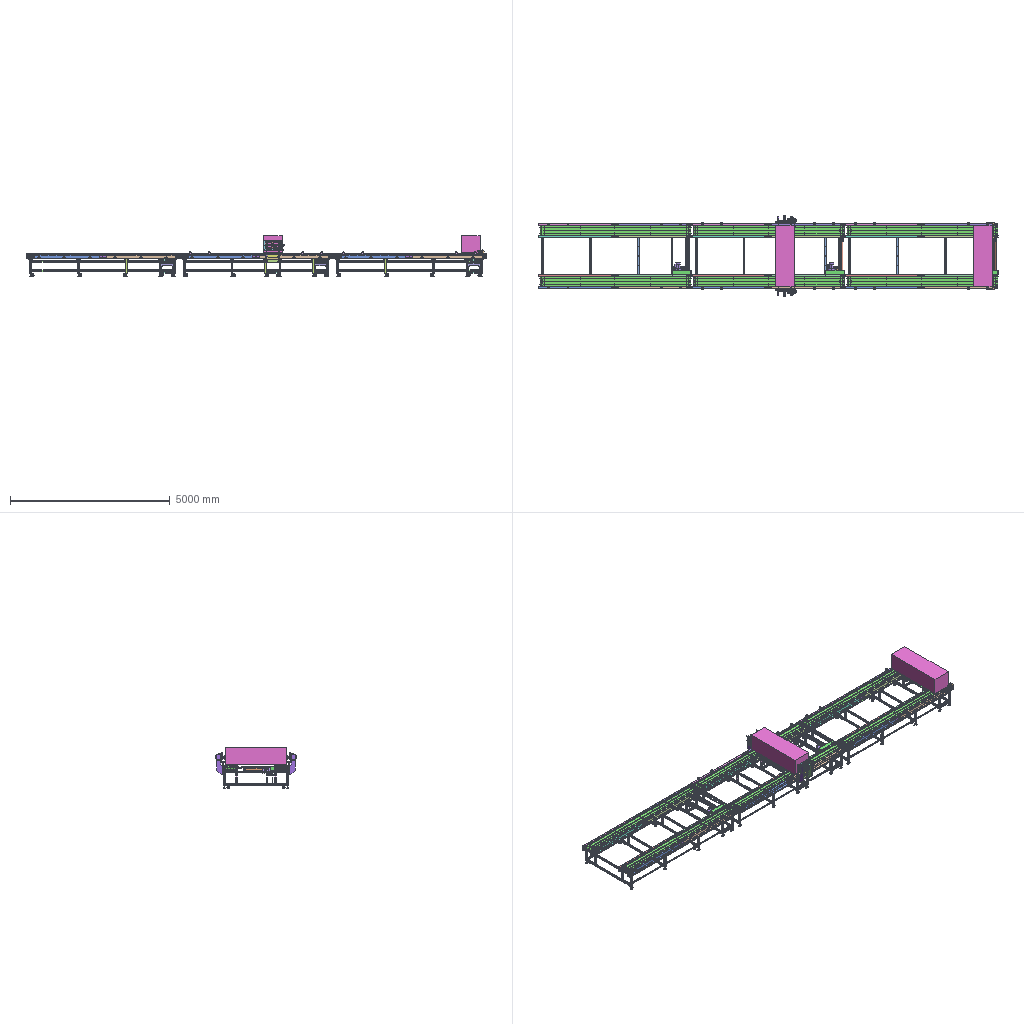Assembly | STEP file | 170 different items | 1185 placed | box 14420 x 2513 x 1274 mm
Parts list (item | name | quantity | parent item | size | volume):
1 | ROLLER.1.stp | x9 | in ROLLER.ASM.stp, ROLLER.ASM.stp-1, TENSION.ROLLER.ASM.stp, ROLLER.ASM.stp-2, ROLLER.ASM.stp-3, TENSION.ROLLER.ASM.stp-1, ROLLER.ASM.stp-4, ROLLER.ASM.stp-5, TENSION.ROLLER.ASM.stp-2 | 114.3 x 130 x 114.3 mm | 316794 mm3
2 | ROLLER.2.stp | x9 | in ROLLER.ASM.stp, ROLLER.ASM.stp-1, TENSION.ROLLER.ASM.stp, ROLLER.ASM.stp-2, ROLLER.ASM.stp-3, TENSION.ROLLER.ASM.stp-1, ROLLER.ASM.stp-4, ROLLER.ASM.stp-5, TENSION.ROLLER.ASM.stp-2 | 114.3 x 130 x 114.3 mm | 316826 mm3
3 | ROLLER.3.stp | x9 | in ROLLER.ASM.stp, ROLLER.ASM.stp-1, TENSION.ROLLER.ASM.stp, ROLLER.ASM.stp-2, ROLLER.ASM.stp-3, TENSION.ROLLER.ASM.stp-1, ROLLER.ASM.stp-4, ROLLER.ASM.stp-5, TENSION.ROLLER.ASM.stp-2 | 114.3 x 90 x 114.3 mm | 702058 mm3
4 | ROLLER.4.stp | x9 | in ROLLER.ASM.stp, ROLLER.ASM.stp-1, TENSION.ROLLER.ASM.stp, ROLLER.ASM.stp-2, ROLLER.ASM.stp-3, TENSION.ROLLER.ASM.stp-1, ROLLER.ASM.stp-4, ROLLER.ASM.stp-5, TENSION.ROLLER.ASM.stp-2 | 100.7 x 12 x 100.7 mm | 87081 mm3
5 | ROLLER.5.stp | x9 | in ROLLER.ASM.stp, ROLLER.ASM.stp-1, TENSION.ROLLER.ASM.stp, ROLLER.ASM.stp-2, ROLLER.ASM.stp-3, TENSION.ROLLER.ASM.stp-1, ROLLER.ASM.stp-4, ROLLER.ASM.stp-5, TENSION.ROLLER.ASM.stp-2 | 100.7 x 12 x 100.7 mm | 87090 mm3
6 | ROLLER.SHAFT.1.stp | x6 | in ROLLER.ASM.stp, ROLLER.ASM.stp-1, ROLLER.ASM.stp-2, ROLLER.ASM.stp-3, ROLLER.ASM.stp-4, ROLLER.ASM.stp-5 | 30 x 504.3 x 30 mm | 316912 mm3
7 | _UCF205 HOUSING.stp | x12 | in UCF205(25,).stp, UCF205(25,).stp-1, UCF205(25,).stp-2, UCF205(25,).stp-3, UCF205(25,).stp-4, UCF205(25,).stp-5, UCF205(25,).stp-6, UCF205(25,).stp-7, UCF205(25,).stp-8, UCF205(25,).stp-9, UCF205(25,).stp-10, UCF205(25,).stp-11 | 95 x 95 x 35.8 mm | 112730 mm3
8 | _BSP50B15-N-25_B.stp | x3 | in BSP50B15-N-25.stp, BSP50B15-N-25.stp-1, BSP50B15-N-25.stp-2 | 83.791 x 83.357 x 25 mm | 63531 mm3
9 | _SET-SCREW8-8.stp | x6 | in BSP50B15-N-25.stp, BSP50B15-N-25.stp-1, BSP50B15-N-25.stp-2 | 8 x 8 x 8 mm | 331.208 mm3
10 | _BSP50B15-N-32_B.stp | x3 | in BSP50B15-N-32.stp, BSP50B15-N-32.stp-1, BSP50B15-N-32.stp-2 | 83.791 x 83.357 x 25 mm | 55752 mm3
11 | _SET-SCREW8-8(2).stp | x6 | in BSP50B15-N-32.stp, BSP50B15-N-32.stp-1, BSP50B15-N-32.stp-2 | 8 x 8 x 8 mm | 331.208 mm3
12 | COUPLING.stp | x6 | in DRIVING.AS.stp, DRIVING.AS.stp-1, DRIVING.AS.stp-2 | 50.056 x 70 x 50.096 mm | 91173 mm3
13 | CONNECTING.SHAFT.stp | x3 | in DRIVING.AS.stp, DRIVING.AS.stp-1, DRIVING.AS.stp-2 | 25 x 1000 x 25 mm | 481905 mm3
14 | ~PA16-150_1.stp | x32 | in ~A-PA-16-150.stp, ~A-PA-16-150.stp-1, ~A-PA-16-150.stp-2, ~A-PA-16-150.stp-3, ~A-PA-16-150.stp-4, ~A-PA-16-150.stp-5, ~A-PA-16-150.stp-6, ~A-PA-16-150.stp-7, ~A-PA-16-150.stp-8, ~A-PA-16-150.stp-9, ~A-PA-16-150.stp-10, ~A-PA-16-150.stp-11, ~A-PA-16-150.stp-12, ~A-PA-16-150.stp-13, ~A-PA-16-150.stp-14, ~A-PA-16-150.stp-15, ~A-PA-16-150.stp-16, ~A-PA-16-150.stp-17, ~A-PA-16-150.stp-18, ~A-PA-16-150.stp-19, ~A-PA-16-150.stp-20, ~A-PA-16-150.stp-21, ~A-PA-16-150.stp-22, ~A-PA-16-150.stp-23, ~A-PA-16-150.stp-24, ~A-PA-16-150.stp-25, ~A-PA-16-150.stp-26, ~A-PA-16-150.stp-27, ~A-PA-16-150.stp-28, ~A-PA-16-150.stp-29, ~A-PA-16-150.stp-30, ~A-PA-16-150.stp-31 | 115 x 75 x 177 mm | 55978 mm3
15 | ~PA16-150_2.stp | x32 | in ~A-PA-16-150.stp, ~A-PA-16-150.stp-1, ~A-PA-16-150.stp-2, ~A-PA-16-150.stp-3, ~A-PA-16-150.stp-4, ~A-PA-16-150.stp-5, ~A-PA-16-150.stp-6, ~A-PA-16-150.stp-7, ~A-PA-16-150.stp-8, ~A-PA-16-150.stp-9, ~A-PA-16-150.stp-10, ~A-PA-16-150.stp-11, ~A-PA-16-150.stp-12, ~A-PA-16-150.stp-13, ~A-PA-16-150.stp-14, ~A-PA-16-150.stp-15, ~A-PA-16-150.stp-16, ~A-PA-16-150.stp-17, ~A-PA-16-150.stp-18, ~A-PA-16-150.stp-19, ~A-PA-16-150.stp-20, ~A-PA-16-150.stp-21, ~A-PA-16-150.stp-22, ~A-PA-16-150.stp-23, ~A-PA-16-150.stp-24, ~A-PA-16-150.stp-25, ~A-PA-16-150.stp-26, ~A-PA-16-150.stp-27, ~A-PA-16-150.stp-28, ~A-PA-16-150.stp-29, ~A-PA-16-150.stp-30, ~A-PA-16-150.stp-31 | 27.7 x 24 x 12 mm | 3543 mm3
16 | ~ACM-600S.stp | x32 | in LEVEL.CASTER.ASM.stp, LEVEL.CASTER.ASM.2.stp, LEVEL.CASTER.ASM.stp-1 | 91.981 x 91 x 90 mm | 300856 mm3
17 | POST.PLATE.1.stp | x16 | in POST.ASM.stp, POST.ASM.stp-1, POST.ASM.stp-2, POST.FRAME.RIGHT.ASM.stp, POST.ASM.stp-3, POST.ASM.stp-4, POST.FRAME.RIGHT.ASM.stp-1, POST.FRAME.MIDDLE.ASM.stp, POST.ASM.stp-5, POST.ASM.stp-6, POST.ASM.stp-7, POST.FRAME.RIGHT.ASM.stp-2 | 120 x 440 x 10 mm | 524955 mm3
18 | POST.PLATE.2.stp | x16 | in POST.ASM.stp, POST.ASM.stp-1, POST.ASM.stp-2, POST.FRAME.RIGHT.ASM.stp, POST.ASM.stp-3, POST.ASM.stp-4, POST.FRAME.RIGHT.ASM.stp-1, POST.FRAME.MIDDLE.ASM.stp, POST.ASM.stp-5, POST.ASM.stp-6, POST.ASM.stp-7, POST.FRAME.RIGHT.ASM.stp-2 | 120 x 440 x 10 mm | 525489 mm3
19 | POST.PLATE.3.stp | x16 | in POST.ASM.stp, POST.ASM.stp-1, POST.ASM.stp-2, POST.FRAME.RIGHT.ASM.stp, POST.ASM.stp-3, POST.ASM.stp-4, POST.FRAME.RIGHT.ASM.stp-1, POST.FRAME.MIDDLE.ASM.stp, POST.ASM.stp-5, POST.ASM.stp-6, POST.ASM.stp-7, POST.FRAME.RIGHT.ASM.stp-2 | 110 x 190 x 10 mm | 131820 mm3
20 | POST.PLATE.4.stp | x16 | in POST.ASM.stp, POST.ASM.stp-1, POST.ASM.stp-2, POST.FRAME.RIGHT.ASM.stp, POST.ASM.stp-3, POST.ASM.stp-4, POST.FRAME.RIGHT.ASM.stp-1, POST.FRAME.MIDDLE.ASM.stp, POST.ASM.stp-5, POST.ASM.stp-6, POST.ASM.stp-7, POST.FRAME.RIGHT.ASM.stp-2 | 110 x 190 x 10 mm | 131820 mm3
21 | POST.SQ.PIPE.1.stp | x16 | in POST.ASM.stp, POST.ASM.stp-1, POST.ASM.stp-2, POST.FRAME.RIGHT.ASM.stp, POST.ASM.stp-3, POST.ASM.stp-4, POST.FRAME.RIGHT.ASM.stp-1, POST.FRAME.MIDDLE.ASM.stp, POST.ASM.stp-5, POST.ASM.stp-6, POST.ASM.stp-7, POST.FRAME.RIGHT.ASM.stp-2 | 50 x 1940 x 50 mm | 1123447 mm3
22 | POST.SQ.PIPE.2.stp | x16 | in POST.ASM.stp, POST.ASM.stp-1, POST.ASM.stp-2, POST.FRAME.RIGHT.ASM.stp, POST.ASM.stp-3, POST.ASM.stp-4, POST.FRAME.RIGHT.ASM.stp-1, POST.FRAME.MIDDLE.ASM.stp, POST.ASM.stp-5, POST.ASM.stp-6, POST.ASM.stp-7, POST.FRAME.RIGHT.ASM.stp-2 | 50 x 1940 x 50 mm | 1123141 mm3
23 | POST.SQ.PIPE.3.stp | x30 | in POST.ASM.stp, POST.ASM.stp-1, POST.ASM.stp-2, POST.FRAME.RIGHT.ASM.stp, POST.ASM.stp-3, POST.ASM.stp-4, POST.FRAME.RIGHT.ASM.stp-1, POST.FRAME.MIDDLE.ASM.stp, POST.ASM.stp-5, POST.ASM.stp-6, POST.ASM.stp-7, POST.FRAME.RIGHT.ASM.stp-2 | 50 x 50 x 440 mm | 254554 mm3
24 | POST.SQ.PIPE.4.stp | x32 | in POST.ASM.stp, POST.ASM.stp-1, POST.ASM.stp-2, POST.FRAME.RIGHT.ASM.stp, POST.ASM.stp-3, POST.ASM.stp-4, POST.FRAME.RIGHT.ASM.stp-1, POST.FRAME.MIDDLE.ASM.stp, POST.ASM.stp-5, POST.ASM.stp-6, POST.ASM.stp-7, POST.FRAME.RIGHT.ASM.stp-2 | 50 x 50 x 340 mm | 196949 mm3
25 | POST.SQ.PIPE.11.stp | x32 | in POST.FRAME.RIGHT.ASM.stp, POST.FRAME.RIGHT.ASM.stp-1, POST.FRAME.MIDDLE.ASM.stp, POST.FRAME.RIGHT.ASM.stp-2 | 50 x 400 x 50 mm | 231705 mm3
26 | MOTOR.PLATE.1.stp | x3 | in POST.FRAME.RIGHT.ASM.stp, POST.FRAME.RIGHT.ASM.stp-1, POST.FRAME.RIGHT.ASM.stp-2 | 340 x 225 x 12 mm | 912612 mm3
27 | MOTOR.RIB.stp | x6 | in POST.FRAME.RIGHT.ASM.stp, POST.FRAME.RIGHT.ASM.stp-1, POST.FRAME.RIGHT.ASM.stp-2 | 440 x 12 x 360 mm | 759276 mm3
28 | LINK.ANGLE.stp | x12 | in LOWER.FRAME.AS.1.stp, LOWER.FRAME.AS.2.stp, LOWER.FRAME.AS.1.stp-1 | 4550 x 50 x 50 mm | 2563197 mm3
29 | ROLLER.SHAFT.IDLE.1.stp | x3 | in TENSION.ROLLER.ASM.stp, TENSION.ROLLER.ASM.stp-1, TENSION.ROLLER.ASM.stp-2 | 30 x 416 x 30 mm | 281205 mm3
30 | _TUUFLN25_B.stp | x6 | in TUUFLN25.stp, TUUFLN25.stp-1, TUUFLN25.stp-2, TUUFLN25.stp-3, TUUFLN25.stp-4, TUUFLN25.stp-5 | 260 x 100 x 27 mm | 84648 mm3
31 | _TUUFLN25_BE.stp | x6 | in TUUFLN25.stp, TUUFLN25.stp-1, TUUFLN25.stp-2, TUUFLN25.stp-3, TUUFLN25.stp-4, TUUFLN25.stp-5 | 28.5 x 85 x 95 mm | 58062 mm3
32 | _SET-SCREW5-7.stp | x12 | in TUUFLN25.stp, TUUFLN25.stp-1, TUUFLN25.stp-2, TUUFLN25.stp-3, TUUFLN25.stp-4, TUUFLN25.stp-5 | 7 x 5 x 5 mm | 119.696 mm3
33 | _TUUFLN25_BO.stp | x6 | in TUUFLN25.stp, TUUFLN25.stp-1, TUUFLN25.stp-2, TUUFLN25.stp-3, TUUFLN25.stp-4, TUUFLN25.stp-5 | 147 x 18.475 x 16 mm | 12547 mm3
34 | _TUUFLN25_N.stp | x12 | in TUUFLN25.stp, TUUFLN25.stp-1, TUUFLN25.stp-2, TUUFLN25.stp-3, TUUFLN25.stp-4, TUUFLN25.stp-5 | 16 x 18.475 x 8 mm | 1314 mm3
35 | MOTOR.BASE.stp | x3 | in MOTOR.UNIT.ASM.stp, MOTOR.UNIT.ASM.stp-1, MOTOR.UNIT.ASM.stp-2 | 235 x 221 x 12 mm | 587706 mm3
36 | BASE.STOPPER.stp | x3 | in MOTOR.UNIT.ASM.stp, MOTOR.UNIT.ASM.stp-1, MOTOR.UNIT.ASM.stp-2 | 15 x 150 x 15 mm | 31025 mm3
37 | ADJUT.BLOCK.stp | x3 | in MOTOR.UNIT.ASM.stp, MOTOR.UNIT.ASM.stp-1, MOTOR.UNIT.ASM.stp-2 | 15 x 150 x 30 mm | 60879 mm3
38 | HEX-HEAD BOLT - KS B 1002 - A M10X80.stp | x6 | in MOTOR.UNIT.ASM.stp, MOTOR.UNIT.ASM.stp-1, MOTOR.UNIT.ASM.stp-2 | 86.4 x 18.48 x 16 mm | 7648 mm3
39 | HEX NUT - KS B 1012 - C M10.stp | x78 | in MOTOR.UNIT.ASM.stp, LINK.BAR.ASM.stp, LINK.BAR.ASM.stp-1, LINK.BAR.ASM.stp-2, LINK.BAR.ASM.stp-3, LINK.BAR.ASM.stp-4, LINK.BAR.ASM.stp-5, LINK.BAR.ASM.stp-6, LINK.BAR.ASM.stp-7, LINK.BAR.ASM.stp-8, LINK.BAR.ASM.stp-9, LINK.BAR.ASM.stp-10, LINK.BAR.ASM.stp-11, LINK.BAR.ASM.stp-12, LINK.BAR.ASM.stp-13, LINK.BAR.ASM.stp-14, LINK.BAR.ASM.stp-15, LINK.BAR.ASM.stp-16, LINK.BAR.ASM.stp-17, LINK.BAR.ASM.stp-18, LINK.BAR.ASM.stp-19, LINK.BAR.ASM.stp-20, LINK.BAR.ASM.stp-21, LINK.BAR.ASM.stp-22, LINK.BAR.ASM.stp-23, MOTOR.UNIT.ASM.stp-1, MOTOR.UNIT.ASM.stp-2, LINK.BAR.ASM.stp-24, LINK.BAR.ASM.stp-25, LINK.BAR.ASM.stp-26, LINK.BAR.ASM.stp-27, LINK.BAR.ASM.stp-28, LINK.BAR.ASM.stp-29, LINK.BAR.ASM.stp-30, LINK.BAR.ASM.stp-31, LINK.BAR.ASM.stp-32, LINK.BAR.ASM.stp-33, LINK.BAR.ASM.stp-34, LINK.BAR.ASM.stp-35 | 9.5 x 18.48 x 16.004 mm | 1564 mm3
40 | M2-135-1_2HP-120HT.stp | x3 | in MOTOR.UNIT.ASM.stp, MOTOR.UNIT.ASM.stp-1, MOTOR.UNIT.ASM.stp-2 | 361 x 214.5 x 237.8 mm | 6497116 mm3
41 | CHAIN.COVER.1.stp | x3 | in MOTOR.UNIT.ASM.stp, MOTOR.UNIT.ASM.stp-1, MOTOR.UNIT.ASM.stp-2 | 600 x 180 x 140 mm | 361793 mm3
42 | CHAIN.COVER.2.stp | x3 | in MOTOR.UNIT.ASM.stp, MOTOR.UNIT.ASM.stp-1, MOTOR.UNIT.ASM.stp-2 | 600 x 2 x 140 mm | 111000 mm3
43 | CHAIN.stp | x3 | in MOTOR.UNIT.ASM.stp, MOTOR.UNIT.ASM.stp-1, MOTOR.UNIT.ASM.stp-2 | 429.35 x 18 x 164.35 mm | 219073 mm3
44 | SPRING WASHER - KS B 1324.stp | x72 | in LINK.BAR.ASM.stp, LINK.BAR.ASM.stp-1, LINK.BAR.ASM.stp-2, LINK.BAR.ASM.stp-3, LINK.BAR.ASM.stp-4, LINK.BAR.ASM.stp-5, LINK.BAR.ASM.stp-6, LINK.BAR.ASM.stp-7, LINK.BAR.ASM.stp-8, LINK.BAR.ASM.stp-9, LINK.BAR.ASM.stp-10, LINK.BAR.ASM.stp-11, LINK.BAR.ASM.stp-12, LINK.BAR.ASM.stp-13, LINK.BAR.ASM.stp-14, LINK.BAR.ASM.stp-15, LINK.BAR.ASM.stp-16, LINK.BAR.ASM.stp-17, LINK.BAR.ASM.stp-18, LINK.BAR.ASM.stp-19, LINK.BAR.ASM.stp-20, LINK.BAR.ASM.stp-21, LINK.BAR.ASM.stp-22, LINK.BAR.ASM.stp-23, LINK.BAR.ASM.stp-24, LINK.BAR.ASM.stp-25, LINK.BAR.ASM.stp-26, LINK.BAR.ASM.stp-27, LINK.BAR.ASM.stp-28, LINK.BAR.ASM.stp-29, LINK.BAR.ASM.stp-30, LINK.BAR.ASM.stp-31, LINK.BAR.ASM.stp-32, LINK.BAR.ASM.stp-33, LINK.BAR.ASM.stp-34, LINK.BAR.ASM.stp-35 | 2.5 x 17.6 x 17.6 mm | 394.643 mm3
45 | PLAIN WASHER REGULAR CIRCULAR - KS B 1326 - 11.stp | x72 | in LINK.BAR.ASM.stp, LINK.BAR.ASM.stp-1, LINK.BAR.ASM.stp-2, LINK.BAR.ASM.stp-3, LINK.BAR.ASM.stp-4, LINK.BAR.ASM.stp-5, LINK.BAR.ASM.stp-6, LINK.BAR.ASM.stp-7, LINK.BAR.ASM.stp-8, LINK.BAR.ASM.stp-9, LINK.BAR.ASM.stp-10, LINK.BAR.ASM.stp-11, LINK.BAR.ASM.stp-12, LINK.BAR.ASM.stp-13, LINK.BAR.ASM.stp-14, LINK.BAR.ASM.stp-15, LINK.BAR.ASM.stp-16, LINK.BAR.ASM.stp-17, LINK.BAR.ASM.stp-18, LINK.BAR.ASM.stp-19, LINK.BAR.ASM.stp-20, LINK.BAR.ASM.stp-21, LINK.BAR.ASM.stp-22, LINK.BAR.ASM.stp-23, LINK.BAR.ASM.stp-24, LINK.BAR.ASM.stp-25, LINK.BAR.ASM.stp-26, LINK.BAR.ASM.stp-27, LINK.BAR.ASM.stp-28, LINK.BAR.ASM.stp-29, LINK.BAR.ASM.stp-30, LINK.BAR.ASM.stp-31, LINK.BAR.ASM.stp-32, LINK.BAR.ASM.stp-33, LINK.BAR.ASM.stp-34, LINK.BAR.ASM.stp-35 | 2 x 21 x 21 mm | 502.655 mm3
46 | _PLSBM17-320-M10-N10.stp | x36 | in LINK.BAR.ASM.stp, LINK.BAR.ASM.stp-1, LINK.BAR.ASM.stp-2, LINK.BAR.ASM.stp-3, LINK.BAR.ASM.stp-4, LINK.BAR.ASM.stp-5, LINK.BAR.ASM.stp-6, LINK.BAR.ASM.stp-7, LINK.BAR.ASM.stp-8, LINK.BAR.ASM.stp-9, LINK.BAR.ASM.stp-10, LINK.BAR.ASM.stp-11, LINK.BAR.ASM.stp-12, LINK.BAR.ASM.stp-13, LINK.BAR.ASM.stp-14, LINK.BAR.ASM.stp-15, LINK.BAR.ASM.stp-16, LINK.BAR.ASM.stp-17, LINK.BAR.ASM.stp-18, LINK.BAR.ASM.stp-19, LINK.BAR.ASM.stp-20, LINK.BAR.ASM.stp-21, LINK.BAR.ASM.stp-22, LINK.BAR.ASM.stp-23, LINK.BAR.ASM.stp-24, LINK.BAR.ASM.stp-25, LINK.BAR.ASM.stp-26, LINK.BAR.ASM.stp-27, LINK.BAR.ASM.stp-28, LINK.BAR.ASM.stp-29, LINK.BAR.ASM.stp-30, LINK.BAR.ASM.stp-31, LINK.BAR.ASM.stp-32, LINK.BAR.ASM.stp-33, LINK.BAR.ASM.stp-34, LINK.BAR.ASM.stp-35 | 366 x 19.63 x 17 mm | 83661 mm3
47 | ROLLER.42.stp | x36 | in BELT.SUPPORT.ROLLER.ASM.stp, BELT.SUPPORT.ROLLER.ASM.stp-1, BELT.SUPPORT.ROLLER.ASM.stp-2, BELT.SUPPORT.ROLLER.ASM.stp-3, BELT.SUPPORT.ROLLER.ASM.stp-4, BELT.SUPPORT.ROLLER.ASM.stp-5, BELT.SUPPORT.ROLLER.ASM.stp-6, BELT.SUPPORT.ROLLER.ASM.stp-7, BELT.SUPPORT.ROLLER.ASM.stp-8, BELT.SUPPORT.ROLLER.ASM.stp-9, BELT.SUPPORT.ROLLER.ASM.stp-10, BELT.SUPPORT.ROLLER.ASM.stp-11, BELT.SUPPORT.ROLLER.ASM.stp-12, BELT.SUPPORT.ROLLER.ASM.stp-13, BELT.SUPPORT.ROLLER.ASM.stp-14, BELT.SUPPORT.ROLLER.ASM.stp-15, BELT.SUPPORT.ROLLER.ASM.stp-16, BELT.SUPPORT.ROLLER.ASM.stp-17, BELT.SUPPORT.ROLLER.ASM.stp-18, BELT.SUPPORT.ROLLER.ASM.stp-19, BELT.SUPPORT.ROLLER.ASM.stp-20, BELT.SUPPORT.ROLLER.ASM.stp-21, BELT.SUPPORT.ROLLER.ASM.stp-22, BELT.SUPPORT.ROLLER.ASM.stp-23, BELT.SUPPORT.ROLLER.ASM.stp-24, BELT.SUPPORT.ROLLER.ASM.stp-25, BELT.SUPPORT.ROLLER.ASM.stp-26, BELT.SUPPORT.ROLLER.ASM.stp-27, BELT.SUPPORT.ROLLER.ASM.stp-28, BELT.SUPPORT.ROLLER.ASM.stp-29, BELT.SUPPORT.ROLLER.ASM.stp-30, BELT.SUPPORT.ROLLER.ASM.stp-31, BELT.SUPPORT.ROLLER.ASM.stp-32, BELT.SUPPORT.ROLLER.ASM.stp-33, BELT.SUPPORT.ROLLER.ASM.stp-34, BELT.SUPPORT.ROLLER.ASM.stp-35 | 43.186 x 318 x 43.662 mm | 413616 mm3
48 | ROLLER.HOLER.stp | x72 | in BELT.SUPPORT.ROLLER.ASM.stp, BELT.SUPPORT.ROLLER.ASM.stp-1, BELT.SUPPORT.ROLLER.ASM.stp-2, BELT.SUPPORT.ROLLER.ASM.stp-3, BELT.SUPPORT.ROLLER.ASM.stp-4, BELT.SUPPORT.ROLLER.ASM.stp-5, BELT.SUPPORT.ROLLER.ASM.stp-6, BELT.SUPPORT.ROLLER.ASM.stp-7, BELT.SUPPORT.ROLLER.ASM.stp-8, BELT.SUPPORT.ROLLER.ASM.stp-9, BELT.SUPPORT.ROLLER.ASM.stp-10, BELT.SUPPORT.ROLLER.ASM.stp-11, BELT.SUPPORT.ROLLER.ASM.stp-12, BELT.SUPPORT.ROLLER.ASM.stp-13, BELT.SUPPORT.ROLLER.ASM.stp-14, BELT.SUPPORT.ROLLER.ASM.stp-15, BELT.SUPPORT.ROLLER.ASM.stp-16, BELT.SUPPORT.ROLLER.ASM.stp-17, BELT.SUPPORT.ROLLER.ASM.stp-18, BELT.SUPPORT.ROLLER.ASM.stp-19, BELT.SUPPORT.ROLLER.ASM.stp-20, BELT.SUPPORT.ROLLER.ASM.stp-21, BELT.SUPPORT.ROLLER.ASM.stp-22, BELT.SUPPORT.ROLLER.ASM.stp-23, BELT.SUPPORT.ROLLER.ASM.stp-24, BELT.SUPPORT.ROLLER.ASM.stp-25, BELT.SUPPORT.ROLLER.ASM.stp-26, BELT.SUPPORT.ROLLER.ASM.stp-27, BELT.SUPPORT.ROLLER.ASM.stp-28, BELT.SUPPORT.ROLLER.ASM.stp-29, BELT.SUPPORT.ROLLER.ASM.stp-30, BELT.SUPPORT.ROLLER.ASM.stp-31, BELT.SUPPORT.ROLLER.ASM.stp-32, BELT.SUPPORT.ROLLER.ASM.stp-33, BELT.SUPPORT.ROLLER.ASM.stp-34, BELT.SUPPORT.ROLLER.ASM.stp-35 | 92 x 10 x 28 mm | 5564 mm3
49 | BELT.PLATE.1.stp | x6 | in BELT.PLATE.ASM.stp, BELT.PLATE.ASM.stp-1, BELT.PLATE.ASM.stp-2 | 1130 x 320 x 43 mm | 956827 mm3
50 | BELT.PLATE.2.stp | x12 | in BELT.PLATE.ASM.stp, BELT.PLATE.ASM.stp-1, BELT.PLATE.ASM.stp-2 | 1150 x 320 x 43 mm | 966060 mm3
51 | BELT.PLATE.12.stp | x6 | in BELT.PLATE.ASM.stp, BELT.PLATE.ASM.stp-1, BELT.PLATE.ASM.stp-2 | 1080 x 320 x 43 mm | 914400 mm3
52 | END.BRACKET.1.stp | x21 | in END.BRACKET.ASM.stp, END.BRACKET.ASM.stp-1, END.BRACKET.ASM.stp-2 | 25 x 50 x 141 mm | 39427 mm3
53 | JOINT.BRACKET.stp | x12 | in UPPER,FRAME.AS.1.stp, UPPER.FRAME.AS.stp, UPPER,FRAME.AS.3.stp | 220 x 55.5 x 141 mm | 210609 mm3
54 | UPPER.FRAME.2.stp | x3 | in UPPER,FRAME.AS.1.stp, UPPER.FRAME.AS.stp, UPPER,FRAME.AS.3.stp | 2400 x 60 x 150 mm | 2791918 mm3
55 | UPPER.FRAME.IDEL.SIDE.2.stp | x3 | in UPPER,FRAME.AS.1.stp, UPPER.FRAME.AS.stp, UPPER,FRAME.AS.3.stp | 2400 x 60 x 150 mm | 2840221 mm3
56 | UPPER.FRAME.IDEL.SIDE.1.stp | x3 | in UPPER,FRAME.AS.1.stp, UPPER.FRAME.AS.stp, UPPER,FRAME.AS.3.stp | 2400 x 60 x 150 mm | 2839315 mm3
57 | UPPER.FRAME.13.stp | x3 | in UPPER,FRAME.AS.1.stp, UPPER.FRAME.AS.stp, UPPER,FRAME.AS.3.stp | 2400 x 60 x 150 mm | 2791917 mm3
58 | UPPER.FRAME.IDLE.SIDE.1.stp | x3 | in UPPER,FRAME.AS.1.stp, UPPER.FRAME.AS.stp, UPPER,FRAME.AS.3.stp | 2400 x 60 x 150 mm | 2839316 mm3
59 | UPPER.FRAME.IDLE.SIDE.2.stp | x3 | in UPPER,FRAME.AS.1.stp, UPPER.FRAME.AS.stp, UPPER,FRAME.AS.3.stp | 2400 x 60 x 150 mm | 2840220 mm3
60 | UPPER.FRAME.1.stp | x3 | in UPPER,FRAME.AS.1.stp, UPPER.FRAME.AS.stp, UPPER,FRAME.AS.3.stp | 2400 x 60 x 150 mm | 2791012 mm3
61 | UPPER.FRAME.12.stp | x3 | in UPPER,FRAME.AS.1.stp, UPPER.FRAME.AS.stp, UPPER,FRAME.AS.3.stp | 2400 x 60 x 150 mm | 2791014 mm3
62 | PVC.BELT.stp | x6 | in BELT.CONVEYOR.AS.1.stp, BELT.CONVEYOR.AS.2.stp, BELT.CONVEYOR.AS.3.stp | 4740 x 300 x 138.65 mm | 11036267 mm3
63 | RIB.1.stp | x2 | in UPPER.FRAME.AS.stp | 12 x 55.5 x 141 mm | 92706 mm3
64 | RIB.2.stp | x2 | in UPPER.FRAME.AS.stp | 12 x 55.5 x 141 mm | 92706 mm3
65 | ATTACH.PLATE.stp | x2 | in UPPER.FRAME.AS.stp | 450 x 12 x 110 mm | 588575 mm3
66 | GUIDE.HOLDER.stp | x16 | in GUIDE.AS.stp, GUIDE.AS.stp-1 | 60 x 62 x 63 mm | 128733 mm3
67 | _CKZT40-X3064L(0)_BODY.stp | x2 | in CKZT40-105T(0).stp, CKZT40-105T(0).stp-1 | 110.5 x 243.9 x 54 mm | 611854 mm3
68 | _CKZT40_ARM.stp | x2 | in CKZT40-105T(0).stp, CKZT40-105T(0).stp-1 | 16 x 16 x 54 mm | 13433 mm3
69 | _CKZT-T040.stp | x2 | in CKZT40-105T(0).stp, CKZT40-105T(0).stp-1 | 75.1 x 22 x 32 mm | 39956 mm3
70 | CLAMP.ARM.1.stp | x4 | in STOPPER.ASM.stp, STOPPER.ASM.stp-1 | 30 x 218 x 11 mm | 63871 mm3
71 | CLAMP.ARM.2.stp | x4 | in STOPPER.ASM.stp, STOPPER.ASM.stp-1 | 16 x 42 x 11 mm | 4382 mm3
72 | CLAMP.ARM.3.stp | x2 | in STOPPER.ASM.stp, STOPPER.ASM.stp-1 | 15 x 70 x 120 mm | 122807 mm3
73 | CENTERING.MOUNT.stp | x2 | in CENTERING.FRAME.ASM.stp, CENTERING.FRAME.ASM2.stp | 450 x 12 x 290 mm | 953602 mm3
74 | CENTERING.RIB.1.stp | x2 | in CENTERING.FRAME.ASM.stp, CENTERING.FRAME.ASM2.stp | 12 x 192 x 666 mm | 1081564 mm3
75 | CENTERING.RIB.2.stp | x2 | in CENTERING.FRAME.ASM.stp, CENTERING.FRAME.ASM2.stp | 12 x 192 x 666 mm | 1019240 mm3
76 | CYL.MOUNT..stp | x1 | in CENTERING.FRAME.ASM.stp | 520 x 12 x 224 mm | 845705 mm3
77 | _CDQ2A50-100-A93(0_0)_BODY.stp | x2 | in CDQ2A50-100DZ-D-A93L(0_0_0).stp, CDQ2A50-100DZ-D-A93L(0_0_0).stp-1 | 140.5 x 71 x 64 mm | 265383 mm3
78 | _CDQ2A50-100-D-A93(0_0)_CYROD.stp | x2 | in CDQ2A50-100DZ-D-A93L(0_0_0).stp, CDQ2A50-100DZ-D-A93L(0_0_0).stp-1 | 123 x 50 x 50 mm | 45835 mm3
79 | _YU-05.stp | x2 | in CDQ2A50-100DZ-D-A93L(0_0_0).stp, CDQ2A50-100DZ-D-A93L(0_0_0).stp-1 | 30 x 19.8 x 19.8 mm | 4960 mm3
80 | _YA-05_CQ2.stp | x2 | in CDQ2A50-100DZ-D-A93L(0_0_0).stp, CDQ2A50-100DZ-D-A93L(0_0_0).stp-1 | 20 x 67 x 20 mm | 14925 mm3
81 | _D-A93(CQ2_50).stp | x4 | in CDQ2A50-100DZ-D-A93L(0_0_0).stp, CDQ2A50-100DZ-D-A93L(0_0_0).stp-1 | 27 x 4.5 x 4 mm | 337.66 mm3
82 | PS16DH.SPM.stp | x4 | in SENSOR.ASM.12.stp, SENSOR.ASM.12.stp-1, SENSOR.ASM.stp, SENSOR.ASM.stp-1 | 60 x 25 x 40 mm | 30010 mm3
83 | PS16UL.SPM.stp | x4 | in SENSOR.ASM.12.stp, SENSOR.ASM.12.stp-1, SENSOR.ASM.stp, SENSOR.ASM.stp-1 | 40 x 26 x 42 mm | 22791 mm3
84 | 16-150.stp | x4 | in SENSOR.ASM.12.stp, SENSOR.ASM.12.stp-1, SENSOR.ASM.stp, SENSOR.ASM.stp-1 | 16 x 16 x 150 mm | 13195 mm3
85 | PUSH.PLATE.stp | x2 | in CENTERING.UNIT.ASM1.stp, CENTERING.UNIT.ASM2.stp | 580 x 12 x 320 mm | 1281951 mm3
86 | CLAMP.PAD.stp | x4 | in CENTERING.UNIT.ASM1.stp, CENTERING.UNIT.ASM2.stp | 50 x 15.025 x 320 mm | 234198 mm3
87 | _LHFSM20.stp | x8 | in CENTERING.UNIT.ASM1.stp, CENTERING.UNIT.ASM2.stp | 42 x 54 x 54 mm | 26319 mm3
88 | _PSFJT20-170-M8(0).stp | x8 | in CENTERING.UNIT.ASM1.stp, CENTERING.UNIT.ASM2.stp | 170 x 20 x 20 mm | 52553 mm3
89 | CYL.MOUNT.2.stp | x1 | in CENTERING.UNIT.ASM2.stp | 520 x 12 x 224 mm | 845706 mm3
90 | POST.SQ.PIPE.31.stp | x2 | in POST.FRAME.MIDDLE.ASM.stp | 50 x 50 x 440 mm | 254875 mm3
91 | ATTACH.PLATE.1.stp | x2 | in POST.FRAME.MIDDLE.ASM.stp | 450 x 12 x 110 mm | 588575 mm3
92 | WORK.1.stp | x2 | in BELT.CONVEYOR.AS.2.stp, BELT.CONVEYOR.AS.3.stp | 587 x 1931 x 541 mm | 613221877 mm3
93 | STOPPER.PAD.stp | x2 | in STOPPER.AS.stp | 15 x 425 x 40 mm | 250251 mm3
94 | STOPPER.BRACKET1.stp | x2 | in STOPPER.AS.stp | 120 x 440 x 140 mm | 215052 mm3
95 | Flange.1.stp | x2 | in Flange.1-Part.stp, Flange.1-Part.stp-1 | 55 x 55 x 8 mm | 12222 mm3
96 | Joint.1.stp | x2 | in Flange.1-Part.stp, Flange.1-Part.stp-1 | 13 x 28 x 28 mm | 4907 mm3
97 | Nut.1.stp | x2 | in Flange.1-Part.stp, Flange.1-Part.stp-1 | 22 x 25.403 x 5 mm | 1177 mm3
98 | Flange.2.stp | x2 | in Flange.2-Part.stp, Flange.2-Part.stp-1 | 55 x 55 x 8 mm | 12222 mm3
99 | Joint.2.stp | x2 | in Flange.2-Part.stp, Flange.2-Part.stp-1 | 13 x 28 x 28 mm | 4907 mm3
100 | Nut.2.stp | x2 | in Flange.2-Part.stp, Flange.2-Part.stp-1 | 22 x 25.403 x 5 mm | 1177 mm3
101 | Flange.3.stp | x2 | in Flange.3-Part.stp, Flange.3-Part.stp-1 | 55 x 55 x 8 mm | 12222 mm3
102 | Joint.3.stp | x2 | in Flange.3-Part.stp, Flange.3-Part.stp-1 | 13 x 28 x 28 mm | 4907 mm3
103 | Nut.3.stp | x2 | in Flange.3-Part.stp, Flange.3-Part.stp-1 | 22 x 25.403 x 5 mm | 1177 mm3
104 | Flange.4.stp | x2 | in Flange.4-Part.stp, Flange.4-Part.stp-1 | 55 x 55 x 8 mm | 12222 mm3
105 | Joint.4.stp | x2 | in Flange.4-Part.stp, Flange.4-Part.stp-1 | 13 x 28 x 28 mm | 4907 mm3
106 | Nut.4.stp | x2 | in Flange.4-Part.stp, Flange.4-Part.stp-1 | 22 x 25.403 x 5 mm | 1177 mm3
107 | LABEL-B.1A.stp | x2 | in RJ05-4SCJ-610X600-100ST_CAPA.stp, RJ05-4SCJ-610X600-100ST_CAPA.stp-1 | 9.877 x 6.344 x 0.16 mm | 5.062 mm3
108 | PART234.stp | x2 | - | 3.09 x 4.487 x 0.1 mm | 0.3955 mm3
109 | PART235.stp | x2 | - | 2.914 x 4.388 x 0.1 mm | 0.3534 mm3
110 | PART242.stp | x2 | - | 2.768 x 4.388 x 0.1 mm | 0.2981 mm3
111 | PART243.stp | x2 | - | 2.692 x 4.487 x 0.1 mm | 0.3611 mm3
112 | PART244.stp | x2 | - | 2.692 x 4.487 x 0.1 mm | 0.3611 mm3
113 | PART245.stp | x2 | - | 1.148 x 4.493 x 0.1 mm | 0.1844 mm3
114 | Bolt.12A.stp | x2 | in Body.1-Part.stp, Body.1-Part.stp-1 | 11 x 11 x 31 mm | 963.854 mm3
115 | Bolt.12AAAAAAAAAAA.stp | x2 | in Body.1-Part.stp, Body.1-Part.stp-1 | 11 x 11 x 31 mm | 963.854 mm3
116 | Bolt.12.stp | x2 | in Body.1-Part.stp, Body.1-Part.stp-1 | 11 x 11 x 31 mm | 963.854 mm3
117 | Gear Box.1(Upper).stp | x2 | in Body.1-Part.stp, Body.1-Part.stp-1 | 65 x 65 x 22 mm | 40348 mm3
118 | Gear Box.1(Lower).stp | x2 | in Body.1-Part.stp, Body.1-Part.stp-1 | 65 x 65 x 28.5 mm | 40735 mm3
119 | LABEL-B.1AAA.stp | x2 | in RJ05-4SCJ-610X600-100ST_CAPAAA.stp, RJ05-4SCJ-610X600-100ST_CAPAAA.stp-1 | 9.877 x 6.344 x 0.16 mm | 5.062 mm3
120 | PART246.stp | x2 | - | 3.09 x 4.487 x 0.1 mm | 0.3955 mm3
121 | PART247.stp | x2 | - | 2.914 x 4.388 x 0.1 mm | 0.3534 mm3
122 | PART248.stp | x2 | - | 2.768 x 4.388 x 0.1 mm | 0.2981 mm3
123 | PART249.stp | x2 | - | 2.692 x 4.487 x 0.1 mm | 0.3611 mm3
124 | PART250.stp | x2 | - | 2.692 x 4.487 x 0.1 mm | 0.3611 mm3
125 | PART251.stp | x2 | - | 1.148 x 4.493 x 0.1 mm | 0.1844 mm3
126 | Bolt.12AA.stp | x2 | in Body.2-Part.stp, Body.2-Part.stp-1 | 11 x 11 x 31 mm | 963.854 mm3
127 | Bolt.12AAAAAAAA.stp | x2 | in Body.2-Part.stp, Body.2-Part.stp-1 | 11 x 11 x 31 mm | 963.854 mm3
128 | Bolt.12AAAAA.stp | x2 | in Body.2-Part.stp, Body.2-Part.stp-1 | 11 x 11 x 31 mm | 963.854 mm3
129 | Gear Box.2(Upper).stp | x2 | in Body.2-Part.stp, Body.2-Part.stp-1 | 65 x 65 x 22 mm | 40348 mm3
130 | Gear Box.2(Lower).stp | x2 | in Body.2-Part.stp, Body.2-Part.stp-1 | 65 x 65 x 28.5 mm | 40735 mm3
131 | LABEL-B.1.stp | x2 | in RJ05-4SCJ-610X600-100ST_CAP.stp, RJ05-4SCJ-610X600-100ST_CAP.stp-1 | 9.877 x 6.344 x 0.16 mm | 5.062 mm3
132 | PART252.stp | x2 | - | 3.09 x 4.487 x 0.1 mm | 0.3955 mm3
133 | PART253.stp | x2 | - | 2.914 x 4.388 x 0.1 mm | 0.3534 mm3
134 | PART254.stp | x2 | - | 2.768 x 4.388 x 0.1 mm | 0.2981 mm3
135 | PART255.stp | x2 | - | 2.692 x 4.487 x 0.1 mm | 0.3611 mm3
136 | PART256.stp | x2 | - | 2.692 x 4.487 x 0.1 mm | 0.3611 mm3
137 | PART257.stp | x2 | - | 1.148 x 4.493 x 0.1 mm | 0.1844 mm3
138 | Bolt.12AAAAAA.stp | x2 | in Body.3-Part.stp, Body.3-Part.stp-1 | 11 x 11 x 31 mm | 963.854 mm3
139 | Bolt.12AAAAAAAAA.stp | x2 | in Body.3-Part.stp, Body.3-Part.stp-1 | 11 x 11 x 31 mm | 963.854 mm3
140 | Bolt.12AAAA.stp | x2 | in Body.3-Part.stp, Body.3-Part.stp-1 | 11 x 11 x 31 mm | 963.854 mm3
141 | Gear Box.3(Upper).stp | x2 | in Body.3-Part.stp, Body.3-Part.stp-1 | 65 x 65 x 22 mm | 40348 mm3
142 | Gear Box.3(Lower).stp | x2 | in Body.3-Part.stp, Body.3-Part.stp-1 | 65 x 65 x 28.5 mm | 40735 mm3
143 | LABEL-B.1AA.stp | x2 | in RJ05-4SCJ-610X600-100ST_CAPAA.stp, RJ05-4SCJ-610X600-100ST_CAPAA.stp-1 | 9.877 x 6.344 x 0.16 mm | 5.062 mm3
144 | PART258.stp | x2 | - | 3.09 x 4.487 x 0.1 mm | 0.3955 mm3
145 | PART259.stp | x2 | - | 2.914 x 4.388 x 0.1 mm | 0.3534 mm3
146 | PART260.stp | x2 | - | 2.768 x 4.388 x 0.1 mm | 0.2981 mm3
147 | PART261.stp | x2 | - | 2.692 x 4.487 x 0.1 mm | 0.3611 mm3
148 | PART262.stp | x2 | - | 2.692 x 4.487 x 0.1 mm | 0.3611 mm3
149 | PART263.stp | x2 | - | 1.148 x 4.493 x 0.1 mm | 0.1844 mm3
150 | Bolt.12AAA.stp | x2 | in Body.4-Part.stp, Body.4-Part.stp-1 | 11 x 11 x 31 mm | 963.854 mm3
151 | Bolt.12AAAAAAA.stp | x2 | in Body.4-Part.stp, Body.4-Part.stp-1 | 11 x 11 x 31 mm | 963.854 mm3
152 | Bolt.12AAAAAAAAAA.stp | x2 | in Body.4-Part.stp, Body.4-Part.stp-1 | 11 x 11 x 31 mm | 963.854 mm3
153 | Gear Box.4(Upper).stp | x2 | in Body.4-Part.stp, Body.4-Part.stp-1 | 65 x 65 x 22 mm | 40348 mm3
154 | Gear Box.4(Lower).stp | x2 | in Body.4-Part.stp, Body.4-Part.stp-1 | 65 x 65 x 28.5 mm | 40735 mm3
155 | Rack Gear(SP-100F).stp | x8 | in SP100F-800X400-100ST.stp, SP100FU-800X300-100ST.stp | 15 x 15 x 165 mm | 27496 mm3
156 | PRODUCT259.stp | x4 | in SP100F-800X400-100ST.stp, SP100FU-800X300-100ST.stp | 10 x 10 x 711 mm | 55834 mm3
157 | - | x2 | in SP100F-800X400-100ST.stp | 10 x 10 x 411 mm | 32272 mm3
158 | _CDQ2F40-50-A93(0_0)_BODY.stp | x2 | in CDQ2F40-50DZ-D-A93(0_0_0).stp, CDQ2F40-50DZ-D-A93(0_0_0).stp-1 | 89.5 x 57 x 52 mm | 126518 mm3
159 | _CDQ2F40-50-D-A93(0_0)_CYROD.stp | x2 | in CDQ2F40-50DZ-D-A93(0_0_0).stp, CDQ2F40-50DZ-D-A93(0_0_0).stp-1 | 82 x 40 x 40 mm | 21214 mm3
160 | _YU-03.stp | x2 | in CDQ2F40-50DZ-D-A93(0_0_0).stp, CDQ2F40-50DZ-D-A93(0_0_0).stp-1 | 28 x 15.8 x 15.8 mm | 2997 mm3
161 | _YA-03_CQ2.stp | x2 | in CDQ2F40-50DZ-D-A93(0_0_0).stp, CDQ2F40-50DZ-D-A93(0_0_0).stp-1 | 18 x 56 x 16 mm | 8735 mm3
162 | _CDQ2F_40().stp | x2 | in CDQ2F40-50DZ-D-A93(0_0_0).stp, CDQ2F40-50DZ-D-A93(0_0_0).stp-1 | 18 x 54 x 72 mm | 25983 mm3
163 | _D-A93(CQ2_40).stp | x4 | in CDQ2F40-50DZ-D-A93(0_0_0).stp, CDQ2F40-50DZ-D-A93(0_0_0).stp-1 | 27 x 4.5 x 4 mm | 337.66 mm3
164 | LIFT.PAD.2.stp | x6 | in LIFTING.UNIT.ASM.1.stp, LIFTING.UNIT.ASM.2.stp | 60 x 880 x 10 mm | 524898 mm3
165 | LIFT.UPPER.PLATE.stp | x1 | in LIFTING.UNIT.ASM.1.stp | 610 x 890 x 30 mm | 2190669 mm3
166 | LOWER.BRACKET.stp | x1 | in LIFTING.UNIT.ASM.1.stp | 582.5 x 770 x 98 mm | 2415812 mm3
167 | SUPPORT.BRACKET.21.stp | x1 | in LIFTING.UNIT.ASM.1.stp | 132.5 x 630 x 92 mm | 804533 mm3
168 | PART2651.stp | x2 | in SP100FU-800X300-100ST.stp | 10 x 10 x 311 mm | 24418 mm3
169 | LIFT.UPPER.PLATE.2.stp | x1 | in LIFTING.UNIT.ASM.2.stp | 610 x 890 x 30 mm | 2296280 mm3
170 | LOWER.BRACKET.2.stp | x1 | in LIFTING.UNIT.ASM.2.stp | 490 x 770 x 98 mm | 2389480 mm3
Placements (level | parent | child | x y z in mm | rotation matrix by rows), first 133 of 1440 lines:
1 | 6.1 | BeltConveyor-1.stp | -0.0 -0.0 -0.0 | 1 0 0 0 1 0 0 0 1
2 | BeltConveyor-1.stp | BELT.CONVEYOR.AS.1.stp | -0.0 -0.0 -0.0 | 1 0 0 0 1 0 0 0 1
3 | BELT.CONVEYOR.AS.1.stp | DRIVING.AS.stp | -10810.0 0.0 2.0 | 1 0 0 0 1 0 0 0 1
4 | DRIVING.AS.stp | ROLLER.ASM.stp | 24474.472 -12453.789 -0.0 | -1 0 0 0 -1 0 0 0 1
5 | ROLLER.ASM.stp | ROLLER.1.stp | 12237.236 -5341.895 75.0 | 1 0 0 0 1 0 0 0 1
5 | ROLLER.ASM.stp | ROLLER.2.stp | 12237.236 -5511.895 75.0 | 1 0 0 0 1 0 0 0 1
5 | ROLLER.ASM.stp | ROLLER.3.stp | 12237.236 -5426.895 75.0 | 1 0 0 0 1 0 0 0 1
5 | ROLLER.ASM.stp | ROLLER.4.stp | 12237.236 -5295.895 75.0 | 1 0 0 0 1 0 0 0 1
5 | ROLLER.ASM.stp | ROLLER.5.stp | 12237.236 -5557.895 75.0 | 1 0 0 0 1 0 0 0 1
5 | ROLLER.ASM.stp | ROLLER.SHAFT.1.stp | 12237.236 -5444.395 75.0 | 1 0 0 0 1 0 0 0 1
4 | DRIVING.AS.stp | ROLLER.ASM.stp-1 | 0.0 -0.0002 -0.0 | 1 0 0 0 1 0 0 0 1
5 | ROLLER.ASM.stp-1 | ROLLER.1.stp | 12237.236 -5341.895 75.0 | 1 0 0 0 1 0 0 0 1
5 | ROLLER.ASM.stp-1 | ROLLER.2.stp | 12237.236 -5511.895 75.0 | 1 0 0 0 1 0 0 0 1
5 | ROLLER.ASM.stp-1 | ROLLER.3.stp | 12237.236 -5426.895 75.0 | 1 0 0 0 1 0 0 0 1
5 | ROLLER.ASM.stp-1 | ROLLER.4.stp | 12237.236 -5295.895 75.0 | 1 0 0 0 1 0 0 0 1
5 | ROLLER.ASM.stp-1 | ROLLER.5.stp | 12237.236 -5557.895 75.0 | 1 0 0 0 1 0 0 0 1
5 | ROLLER.ASM.stp-1 | ROLLER.SHAFT.1.stp | 12237.236 -5444.395 75.0 | 1 0 0 0 1 0 0 0 1
4 | DRIVING.AS.stp | UCF205(25,).stp | 12237.236 -5600.395 75.0 | 1 0 0 0 0 -1 0 1 0
5 | UCF205(25,).stp | _UCF205 HOUSING.stp | -0.0 -0.0 -0.0 | 1 0 0 0 1 0 0 0 1
4 | DRIVING.AS.stp | UCF205(25,).stp-1 | 12237.236 -5253.395 75.0 | -1 0 0 0 0 1 0 1 0
5 | UCF205(25,).stp-1 | _UCF205 HOUSING.stp | -0.0 -0.0 -0.0 | 1 0 0 0 1 0 0 0 1
4 | DRIVING.AS.stp | UCF205(25,).stp-2 | 12237.236 -7200.395 75.0 | 1 0 0 0 0 -1 0 1 0
5 | UCF205(25,).stp-2 | _UCF205 HOUSING.stp | -0.0 -0.0 -0.0 | 1 0 0 0 1 0 0 0 1
4 | DRIVING.AS.stp | UCF205(25,).stp-3 | 12237.236 -6853.395 75.0 | -1 0 0 0 0 1 0 1 0
5 | UCF205(25,).stp-3 | _UCF205 HOUSING.stp | -0.0 -0.0 -0.0 | 1 0 0 0 1 0 0 0 1
4 | DRIVING.AS.stp | BSP50B15-N-25.stp | 12237.236 -6772.595 75.0 | 1 0 0 0 0 -1 0 1 0
5 | BSP50B15-N-25.stp | _BSP50B15-N-25_B.stp | -0.0 -0.0 -0.0 | 1 0 0 0 1 0 0 0 1
5 | BSP50B15-N-25.stp | _SET-SCREW8-8.stp | 10.825 -6.25 18.0 | -0.866 0 0.5 0.5 0 0.866 0 1 0
5 | BSP50B15-N-25.stp | _SET-SCREW8-8.stp | -0.0 15.8 18.0 | 0 0 -1 -1 0 0 0 1 0
4 | DRIVING.AS.stp | BSP50B15-N-32.stp | 11897.236 -6781.295 0.0 | -1 0 0 0 0 1 0 1 0
5 | BSP50B15-N-32.stp | _BSP50B15-N-32_B.stp | -0.0 -0.0 -0.0 | 1 0 0 0 1 0 0 0 1
5 | BSP50B15-N-32.stp | _SET-SCREW8-8(2).stp | -0.0 19.3 18.0 | 0 0 -1 -1 0 0 0 1 0
5 | BSP50B15-N-32.stp | _SET-SCREW8-8(2).stp | 13.856 -8.0 18.0 | -0.866 0 0.5 0.5 0 0.866 0 1 0
4 | DRIVING.AS.stp | COUPLING.stp | 12237.236 -6726.895 75.0 | 1 0 0 0 1 0 0 0 1
4 | DRIVING.AS.stp | COUPLING.stp | 12237.236 -5726.895 75.0 | 1 0 0 0 1 0 0 0 1
4 | DRIVING.AS.stp | CONNECTING.SHAFT.stp | 12237.236 -6226.895 75.0 | 1 0 0 0 1 0 0 0 1
3 | BELT.CONVEYOR.AS.1.stp | LEVEL.CASTER.ASM.stp | -10810.0 0.0 -0.0 | 1 0 0 0 1 0 0 0 1
4 | LEVEL.CASTER.ASM.stp | ~A-PA-16-150.stp | 15323.86 -13222.691 -2611.426 | -1 0 0 0 -1 0 0 0 1
5 | ~A-PA-16-150.stp | ~PA16-150_1.stp | 3186.624 -6000.797 2132.926 | 1 0 0 0 1 0 0 0 1
5 | ~A-PA-16-150.stp | ~PA16-150_2.stp | 3166.624 -6000.797 2128.426 | 1 0 0 0 1 0 0 0 1
4 | LEVEL.CASTER.ASM.stp | ~A-PA-16-150.stp-1 | 15323.86 -11232.691 -2611.426 | -1 0 0 0 -1 0 0 0 1
5 | ~A-PA-16-150.stp-1 | ~PA16-150_1.stp | 3186.624 -6000.797 2132.926 | 1 0 0 0 1 0 0 0 1
5 | ~A-PA-16-150.stp-1 | ~PA16-150_2.stp | 3166.624 -6000.797 2128.426 | 1 0 0 0 1 0 0 0 1
4 | LEVEL.CASTER.ASM.stp | ~A-PA-16-150.stp-2 | 13823.86 -13222.691 -2611.426 | -1 0 0 0 -1 0 0 0 1
5 | ~A-PA-16-150.stp-2 | ~PA16-150_1.stp | 3186.624 -6000.797 2132.926 | 1 0 0 0 1 0 0 0 1
5 | ~A-PA-16-150.stp-2 | ~PA16-150_2.stp | 3166.624 -6000.797 2128.426 | 1 0 0 0 1 0 0 0 1
4 | LEVEL.CASTER.ASM.stp | ~A-PA-16-150.stp-3 | 5990.612 -1221.098 -2611.426 | 1 0 0 0 1 0 0 0 1
5 | ~A-PA-16-150.stp-3 | ~PA16-150_1.stp | 3186.624 -6000.797 2132.926 | 1 0 0 0 1 0 0 0 1
5 | ~A-PA-16-150.stp-3 | ~PA16-150_2.stp | 3166.624 -6000.797 2128.426 | 1 0 0 0 1 0 0 0 1
4 | LEVEL.CASTER.ASM.stp | ~A-PA-16-150.stp-4 | 4490.612 -1221.098 -2611.426 | 1 0 0 0 1 0 0 0 1
5 | ~A-PA-16-150.stp-4 | ~PA16-150_1.stp | 3186.624 -6000.797 2132.926 | 1 0 0 0 1 0 0 0 1
5 | ~A-PA-16-150.stp-4 | ~PA16-150_2.stp | 3166.624 -6000.797 2128.426 | 1 0 0 0 1 0 0 0 1
4 | LEVEL.CASTER.ASM.stp | ~A-PA-16-150.stp-5 | 4490.612 768.902 -2611.426 | 1 0 0 0 1 0 0 0 1
5 | ~A-PA-16-150.stp-5 | ~PA16-150_1.stp | 3186.624 -6000.797 2132.926 | 1 0 0 0 1 0 0 0 1
5 | ~A-PA-16-150.stp-5 | ~PA16-150_2.stp | 3166.624 -6000.797 2128.426 | 1 0 0 0 1 0 0 0 1
4 | LEVEL.CASTER.ASM.stp | ~A-PA-16-150.stp-6 | 13823.86 -11232.691 -2611.426 | -1 0 0 0 -1 0 0 0 1
5 | ~A-PA-16-150.stp-6 | ~PA16-150_1.stp | 3186.624 -6000.797 2132.926 | 1 0 0 0 1 0 0 0 1
5 | ~A-PA-16-150.stp-6 | ~PA16-150_2.stp | 3166.624 -6000.797 2128.426 | 1 0 0 0 1 0 0 0 1
4 | LEVEL.CASTER.ASM.stp | ~A-PA-16-150.stp-7 | 5990.612 768.902 -2611.426 | 1 0 0 0 1 0 0 0 1
5 | ~A-PA-16-150.stp-7 | ~PA16-150_1.stp | 3186.624 -6000.797 2132.926 | 1 0 0 0 1 0 0 0 1
5 | ~A-PA-16-150.stp-7 | ~PA16-150_2.stp | 3166.624 -6000.797 2128.426 | 1 0 0 0 1 0 0 0 1
4 | LEVEL.CASTER.ASM.stp | ~A-PA-16-150.stp-8 | 8540.612 -1221.098 -2611.426 | 1 0 0 0 1 0 0 0 1
5 | ~A-PA-16-150.stp-8 | ~PA16-150_1.stp | 3186.624 -6000.797 2132.926 | 1 0 0 0 1 0 0 0 1
5 | ~A-PA-16-150.stp-8 | ~PA16-150_2.stp | 3166.624 -6000.797 2128.426 | 1 0 0 0 1 0 0 0 1
4 | LEVEL.CASTER.ASM.stp | ~A-PA-16-150.stp-9 | 8540.612 768.902 -2611.426 | 1 0 0 0 1 0 0 0 1
5 | ~A-PA-16-150.stp-9 | ~PA16-150_1.stp | 3186.624 -6000.797 2132.926 | 1 0 0 0 1 0 0 0 1
5 | ~A-PA-16-150.stp-9 | ~PA16-150_2.stp | 3166.624 -6000.797 2128.426 | 1 0 0 0 1 0 0 0 1
4 | LEVEL.CASTER.ASM.stp | ~ACM-600S.stp | 12093.926 -5361.895 -526.31 | -1 0 0 0 -1 0 0 0 1
4 | LEVEL.CASTER.ASM.stp | ~ACM-600S.stp | 10593.926 -7091.895 -526.31 | -1 0 0 0 -1 0 0 0 1
4 | LEVEL.CASTER.ASM.stp | ~ACM-600S.stp | 10593.926 -5361.895 -526.31 | -1 0 0 0 -1 0 0 0 1
4 | LEVEL.CASTER.ASM.stp | ~ACM-600S.stp | 9220.546 -7091.895 -526.31 | 1 0 0 0 1 0 0 0 1
4 | LEVEL.CASTER.ASM.stp | ~ACM-600S.stp | 9220.546 -5361.895 -526.31 | 1 0 0 0 1 0 0 0 1
4 | LEVEL.CASTER.ASM.stp | ~ACM-600S.stp | 12093.926 -7091.895 -526.31 | -1 0 0 0 -1 0 0 0 1
4 | LEVEL.CASTER.ASM.stp | ~ACM-600S.stp | 11770.546 -7091.895 -526.31 | 1 0 0 0 1 0 0 0 1
4 | LEVEL.CASTER.ASM.stp | ~ACM-600S.stp | 11770.546 -5361.895 -526.31 | 1 0 0 0 1 0 0 0 1
4 | LEVEL.CASTER.ASM.stp | ~ACM-600S.stp | 7720.546 -7091.895 -526.31 | 1 0 0 0 1 0 0 0 1
4 | LEVEL.CASTER.ASM.stp | ~ACM-600S.stp | 7720.546 -5361.895 -526.31 | 1 0 0 0 1 0 0 0 1
3 | BELT.CONVEYOR.AS.1.stp | LOWER.FRAME.AS.1.stp | -10810.0 0.0 -0.0 | 1 0 0 0 1 0 0 0 1
4 | LOWER.FRAME.AS.1.stp | POST.ASM.stp | -1500.0 -0.0 -0.0 | 1 0 0 0 1 0 0 0 1
5 | POST.ASM.stp | POST.PLATE.1.stp | 12157.236 -7026.895 -22.0 | 1 0 0 0 1 0 0 0 1
5 | POST.ASM.stp | POST.PLATE.2.stp | 12157.236 -5426.895 -22.0 | 1 0 0 0 1 0 0 0 1
5 | POST.ASM.stp | POST.PLATE.3.stp | 12127.236 -7151.895 -472.0 | 1 0 0 0 1 0 0 0 1
5 | POST.ASM.stp | POST.PLATE.4.stp | 12127.236 -5301.895 -472.0 | 1 0 0 0 1 0 0 0 1
5 | POST.ASM.stp | POST.SQ.PIPE.1.stp | 12157.236 -6226.895 -442.0 | 1 0 0 0 1 0 0 0 1
5 | POST.ASM.stp | POST.SQ.PIPE.2.stp | 12157.236 -6226.895 -52.0 | 1 0 0 0 1 0 0 0 1
5 | POST.ASM.stp | POST.SQ.PIPE.3.stp | 12157.236 -5231.895 -247.0 | 1 0 0 0 1 0 0 0 1
5 | POST.ASM.stp | POST.SQ.PIPE.3.stp | 12157.236 -7221.895 -247.0 | -1 0 0 0 -1 0 0 0 1
5 | POST.ASM.stp | POST.SQ.PIPE.4.stp | 12157.236 -6831.895 -247.0 | 1 0 0 0 1 0 0 0 1
5 | POST.ASM.stp | POST.SQ.PIPE.4.stp | 12157.236 -5621.895 -247.0 | 1 0 0 0 1 0 0 0 1
4 | LOWER.FRAME.AS.1.stp | POST.ASM.stp-1 | 21314.472 -12453.789 -0.0 | -1 0 0 0 -1 0 0 0 1
5 | POST.ASM.stp-1 | POST.PLATE.1.stp | 12157.236 -7026.895 -22.0 | 1 0 0 0 1 0 0 0 1
5 | POST.ASM.stp-1 | POST.PLATE.2.stp | 12157.236 -5426.895 -22.0 | 1 0 0 0 1 0 0 0 1
5 | POST.ASM.stp-1 | POST.PLATE.3.stp | 12127.236 -7151.895 -472.0 | 1 0 0 0 1 0 0 0 1
5 | POST.ASM.stp-1 | POST.PLATE.4.stp | 12127.236 -5301.895 -472.0 | 1 0 0 0 1 0 0 0 1
5 | POST.ASM.stp-1 | POST.SQ.PIPE.1.stp | 12157.236 -6226.895 -442.0 | 1 0 0 0 1 0 0 0 1
5 | POST.ASM.stp-1 | POST.SQ.PIPE.2.stp | 12157.236 -6226.895 -52.0 | 1 0 0 0 1 0 0 0 1
5 | POST.ASM.stp-1 | POST.SQ.PIPE.3.stp | 12157.236 -5231.895 -247.0 | 1 0 0 0 1 0 0 0 1
5 | POST.ASM.stp-1 | POST.SQ.PIPE.3.stp | 12157.236 -7221.895 -247.0 | -1 0 0 0 -1 0 0 0 1
5 | POST.ASM.stp-1 | POST.SQ.PIPE.4.stp | 12157.236 -5621.895 -247.0 | 1 0 0 0 1 0 0 0 1
5 | POST.ASM.stp-1 | POST.SQ.PIPE.4.stp | 12157.236 -6831.895 -247.0 | 1 0 0 0 1 0 0 0 1
4 | LOWER.FRAME.AS.1.stp | POST.ASM.stp-2 | 19814.472 -12453.789 -0.0 | -1 0 0 0 -1 0 0 0 1
5 | POST.ASM.stp-2 | POST.PLATE.1.stp | 12157.236 -7026.895 -22.0 | 1 0 0 0 1 0 0 0 1
5 | POST.ASM.stp-2 | POST.PLATE.2.stp | 12157.236 -5426.895 -22.0 | 1 0 0 0 1 0 0 0 1
5 | POST.ASM.stp-2 | POST.PLATE.3.stp | 12127.236 -7151.895 -472.0 | 1 0 0 0 1 0 0 0 1
5 | POST.ASM.stp-2 | POST.PLATE.4.stp | 12127.236 -5301.895 -472.0 | 1 0 0 0 1 0 0 0 1
5 | POST.ASM.stp-2 | POST.SQ.PIPE.1.stp | 12157.236 -6226.895 -442.0 | 1 0 0 0 1 0 0 0 1
5 | POST.ASM.stp-2 | POST.SQ.PIPE.2.stp | 12157.236 -6226.895 -52.0 | 1 0 0 0 1 0 0 0 1
5 | POST.ASM.stp-2 | POST.SQ.PIPE.3.stp | 12157.236 -7221.895 -247.0 | -1 0 0 0 -1 0 0 0 1
5 | POST.ASM.stp-2 | POST.SQ.PIPE.3.stp | 12157.236 -5231.895 -247.0 | 1 0 0 0 1 0 0 0 1
5 | POST.ASM.stp-2 | POST.SQ.PIPE.4.stp | 12157.236 -6831.895 -247.0 | 1 0 0 0 1 0 0 0 1
5 | POST.ASM.stp-2 | POST.SQ.PIPE.4.stp | 12157.236 -5621.895 -247.0 | 1 0 0 0 1 0 0 0 1
4 | LOWER.FRAME.AS.1.stp | POST.FRAME.RIGHT.ASM.stp | 6000.0 -0.0 -0.0 | 1 0 0 0 1 0 0 0 1
5 | POST.FRAME.RIGHT.ASM.stp | POST.PLATE.1.stp | 6157.236 -7026.895 -22.0 | 1 0 0 0 1 0 0 0 1
5 | POST.FRAME.RIGHT.ASM.stp | POST.PLATE.1.stp | 5707.236 -5426.895 -22.0 | -1 0 0 0 -1 0 0 0 1
5 | POST.FRAME.RIGHT.ASM.stp | POST.PLATE.2.stp | 5707.236 -7026.895 -22.0 | -1 0 0 0 -1 0 0 0 1
5 | POST.FRAME.RIGHT.ASM.stp | POST.PLATE.2.stp | 6157.236 -5426.895 -22.0 | 1 0 0 0 1 0 0 0 1
5 | POST.FRAME.RIGHT.ASM.stp | POST.PLATE.3.stp | 6127.236 -7151.895 -472.0 | 1 0 0 0 1 0 0 0 1
5 | POST.FRAME.RIGHT.ASM.stp | POST.PLATE.3.stp | 5737.236 -5301.895 -472.0 | -1 0 0 0 -1 0 0 0 1
5 | POST.FRAME.RIGHT.ASM.stp | POST.PLATE.4.stp | 6127.236 -5301.895 -472.0 | 1 0 0 0 1 0 0 0 1
5 | POST.FRAME.RIGHT.ASM.stp | POST.PLATE.4.stp | 5737.236 -7151.895 -472.0 | -1 0 0 0 -1 0 0 0 1
5 | POST.FRAME.RIGHT.ASM.stp | POST.SQ.PIPE.1.stp | 5707.236 -6226.895 -442.0 | -1 0 0 0 -1 0 0 0 1
5 | POST.FRAME.RIGHT.ASM.stp | POST.SQ.PIPE.1.stp | 6157.236 -6226.895 -442.0 | 1 0 0 0 1 0 0 0 1
5 | POST.FRAME.RIGHT.ASM.stp | POST.SQ.PIPE.2.stp | 6157.236 -6226.895 -52.0 | 1 0 0 0 1 0 0 0 1
5 | POST.FRAME.RIGHT.ASM.stp | POST.SQ.PIPE.2.stp | 5707.236 -6226.895 -52.0 | -1 0 0 0 -1 0 0 0 1
5 | POST.FRAME.RIGHT.ASM.stp | POST.SQ.PIPE.3.stp | 6157.236 -7221.895 -247.0 | -1 0 0 0 -1 0 0 0 1
5 | POST.FRAME.RIGHT.ASM.stp | POST.SQ.PIPE.3.stp | 5707.236 -5231.895 -247.0 | 1 0 0 0 1 0 0 0 1
5 | POST.FRAME.RIGHT.ASM.stp | POST.SQ.PIPE.3.stp | 6157.236 -5231.895 -247.0 | 1 0 0 0 1 0 0 0 1
5 | POST.FRAME.RIGHT.ASM.stp | POST.SQ.PIPE.3.stp | 5707.236 -7221.895 -247.0 | -1 0 0 0 -1 0 0 0 1
5 | POST.FRAME.RIGHT.ASM.stp | POST.SQ.PIPE.4.stp | 5707.236 -6831.895 -247.0 | -1 0 0 0 -1 0 0 0 1
5 | POST.FRAME.RIGHT.ASM.stp | POST.SQ.PIPE.4.stp | 6157.236 -6831.895 -247.0 | 1 0 0 0 1 0 0 0 1
5 | POST.FRAME.RIGHT.ASM.stp | POST.SQ.PIPE.4.stp | 6157.236 -5621.895 -247.0 | 1 0 0 0 1 0 0 0 1
5 | POST.FRAME.RIGHT.ASM.stp | POST.SQ.PIPE.4.stp | 5707.236 -5621.895 -247.0 | -1 0 0 0 -1 0 0 0 1
5 | POST.FRAME.RIGHT.ASM.stp | POST.SQ.PIPE.11.stp | 6502.236 -6831.895 -52.0 | 0 -1 0 1 0 0 0 0 1